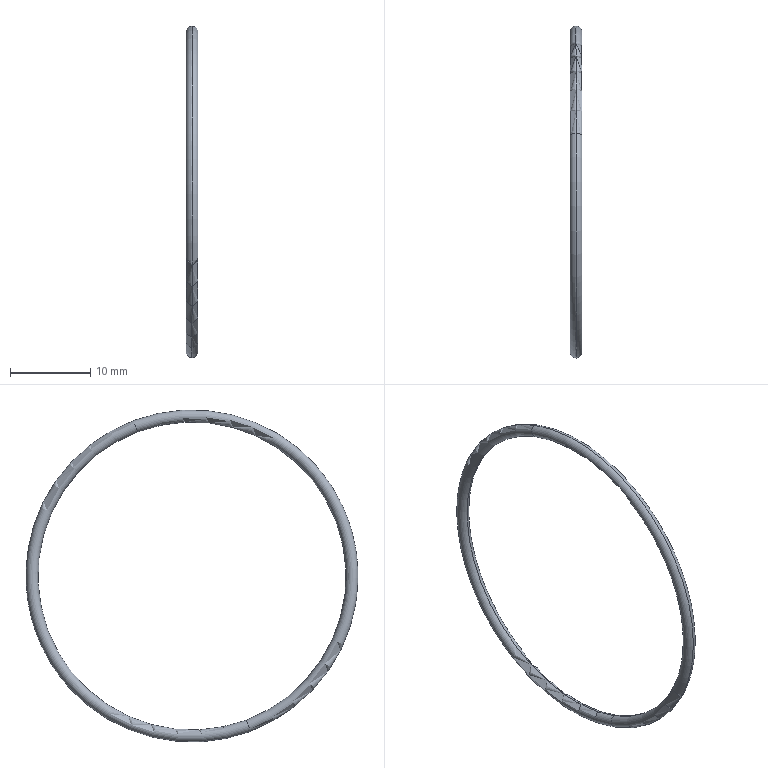Part | SolidWorks | features BaseBody 1 | 1 solid | 4 faces | box 1.5 x 41.5 x 41.5 mm | volume 222.066 mm3 | torus 4
STEP:
#1=CARTESIAN_POINT('',(-7.3,-7.301,-19.423));
#2=VERTEX_POINT('',#1);
#3=CARTESIAN_POINT('',(-7.3,-6.773,-18.019));
#4=VERTEX_POINT('',#3);
#5=CARTESIAN_POINT('',(-7.3,-7.037,-18.721));
#6=DIRECTION('',(0.,-0.9361,0.3518));
#7=DIRECTION('',(0.,-0.3518,-0.9361));
#8=AXIS2_PLACEMENT_3D('',#5,#6,#7);
#9=CIRCLE('',#8,0.75);
#10=EDGE_CURVE('',#2,#4,#9,.T.);
#11=ORIENTED_EDGE('',*,*,#10,.F.);
#12=CARTESIAN_POINT('',(-7.3,7.301,19.423));
#13=VERTEX_POINT('',#12);
#14=CARTESIAN_POINT('',(-7.3,0.,0.));
#15=DIRECTION('',(1.,0.,0.));
#16=DIRECTION('',(0.,0.,-1.));
#17=AXIS2_PLACEMENT_3D('',#14,#15,#16);
#18=CIRCLE('',#17,20.75);
#19=EDGE_CURVE('',#2,#13,#18,.T.);
#20=ORIENTED_EDGE('',*,*,#19,.T.);
#21=CARTESIAN_POINT('',(-7.3,6.773,18.019));
#22=VERTEX_POINT('',#21);
#23=CARTESIAN_POINT('',(-7.3,7.037,18.721));
#24=DIRECTION('',(0.,0.9361,-0.3518));
#25=DIRECTION('',(0.,0.3518,0.9361));
#26=AXIS2_PLACEMENT_3D('',#23,#24,#25);
#27=CIRCLE('',#26,0.75);
#28=EDGE_CURVE('',#13,#22,#27,.T.);
#29=ORIENTED_EDGE('',*,*,#28,.T.);
#30=CARTESIAN_POINT('',(-7.3,0.,0.));
#31=DIRECTION('',(1.,0.,0.));
#32=DIRECTION('',(0.,0.,-1.));
#33=AXIS2_PLACEMENT_3D('',#30,#31,#32);
#34=CIRCLE('',#33,19.25);
#35=EDGE_CURVE('',#4,#22,#34,.T.);
#36=ORIENTED_EDGE('',*,*,#35,.F.);
#37=EDGE_LOOP('',(#11,#20,#29,#36));
#38=FACE_OUTER_BOUND('',#37,.T.);
#39=CARTESIAN_POINT('',(-7.3,0.,0.));
#40=DIRECTION('',(1.,0.,0.));
#41=DIRECTION('',(0.,0.3518,0.9361));
#42=AXIS2_PLACEMENT_3D('',#39,#40,#41);
#43=TOROIDAL_SURFACE('',#42,20.,0.75);
#44=ADVANCED_FACE('',(#38),#43,.T.);
#45=ORIENTED_EDGE('',*,*,#28,.F.);
#46=CARTESIAN_POINT('',(-7.3,0.,0.));
#47=DIRECTION('',(1.,0.,0.));
#48=DIRECTION('',(0.,0.,-1.));
#49=AXIS2_PLACEMENT_3D('',#46,#47,#48);
#50=CIRCLE('',#49,20.75);
#51=EDGE_CURVE('',#13,#2,#50,.T.);
#52=ORIENTED_EDGE('',*,*,#51,.T.);
#53=ORIENTED_EDGE('',*,*,#10,.T.);
#54=CARTESIAN_POINT('',(-7.3,0.,0.));
#55=DIRECTION('',(1.,0.,0.));
#56=DIRECTION('',(0.,0.,-1.));
#57=AXIS2_PLACEMENT_3D('',#54,#55,#56);
#58=CIRCLE('',#57,19.25);
#59=EDGE_CURVE('',#22,#4,#58,.T.);
#60=ORIENTED_EDGE('',*,*,#59,.F.);
#61=EDGE_LOOP('',(#45,#52,#53,#60));
#62=FACE_OUTER_BOUND('',#61,.T.);
#63=CARTESIAN_POINT('',(-7.3,0.,0.));
#64=DIRECTION('',(1.,0.,0.));
#65=DIRECTION('',(0.,0.3518,0.9361));
#66=AXIS2_PLACEMENT_3D('',#63,#64,#65);
#67=TOROIDAL_SURFACE('',#66,20.,0.75);
#68=ADVANCED_FACE('',(#62),#67,.T.);
#69=ORIENTED_EDGE('',*,*,#51,.F.);
#70=CARTESIAN_POINT('',(-7.3,7.037,18.721));
#71=DIRECTION('',(0.,0.9361,-0.3518));
#72=DIRECTION('',(0.,0.3518,0.9361));
#73=AXIS2_PLACEMENT_3D('',#70,#71,#72);
#74=CIRCLE('',#73,0.75);
#75=EDGE_CURVE('',#22,#13,#74,.T.);
#76=ORIENTED_EDGE('',*,*,#75,.F.);
#77=ORIENTED_EDGE('',*,*,#59,.T.);
#78=CARTESIAN_POINT('',(-7.3,-7.037,-18.721));
#79=DIRECTION('',(0.,-0.9361,0.3518));
#80=DIRECTION('',(0.,-0.3518,-0.9361));
#81=AXIS2_PLACEMENT_3D('',#78,#79,#80);
#82=CIRCLE('',#81,0.75);
#83=EDGE_CURVE('',#4,#2,#82,.T.);
#84=ORIENTED_EDGE('',*,*,#83,.T.);
#85=EDGE_LOOP('',(#69,#76,#77,#84));
#86=FACE_OUTER_BOUND('',#85,.T.);
#87=CARTESIAN_POINT('',(-7.3,0.,0.));
#88=DIRECTION('',(1.,0.,0.));
#89=DIRECTION('',(0.,0.3518,0.9361));
#90=AXIS2_PLACEMENT_3D('',#87,#88,#89);
#91=TOROIDAL_SURFACE('',#90,20.,0.75);
#92=ADVANCED_FACE('',(#86),#91,.T.);
#93=ORIENTED_EDGE('',*,*,#19,.F.);
#94=ORIENTED_EDGE('',*,*,#83,.F.);
#95=ORIENTED_EDGE('',*,*,#35,.T.);
#96=ORIENTED_EDGE('',*,*,#75,.T.);
#97=EDGE_LOOP('',(#93,#94,#95,#96));
#98=FACE_OUTER_BOUND('',#97,.T.);
#99=CARTESIAN_POINT('',(-7.3,0.,0.));
#100=DIRECTION('',(1.,0.,0.));
#101=DIRECTION('',(0.,0.3518,0.9361));
#102=AXIS2_PLACEMENT_3D('',#99,#100,#101);
#103=TOROIDAL_SURFACE('',#102,20.,0.75);
#104=ADVANCED_FACE('',(#98),#103,.T.);
#105=CLOSED_SHELL('',(#44,#68,#92,#104));
#106=MANIFOLD_SOLID_BREP('',#105);
#107=CARTESIAN_POINT('',(0.,0.,0.));
#108=DIRECTION('',(0.,0.,1.));
#109=DIRECTION('',(1.,0.,0.));
#110=AXIS2_PLACEMENT_3D('',#107,#108,#109);
#111=(LENGTH_UNIT()NAMED_UNIT(*)SI_UNIT(.MILLI.,.METRE.));
#112=UNCERTAINTY_MEASURE_WITH_UNIT(LENGTH_MEASURE(0.00001),#111,'','');
#113=(NAMED_UNIT(*)PLANE_ANGLE_UNIT()SI_UNIT($,.RADIAN.));
#114=(NAMED_UNIT(*)SI_UNIT($,.STERADIAN.)SOLID_ANGLE_UNIT());
#115=(GEOMETRIC_REPRESENTATION_CONTEXT(3)GLOBAL_UNCERTAINTY_ASSIGNED_CONTEXT((#112))GLOBAL_UNIT_ASSIGNED_CONTEXT((#111,#113,#114))REPRESENTATION_CONTEXT('',''));
#116=ADVANCED_BREP_SHAPE_REPRESENTATION('',(#106,#110),#115);